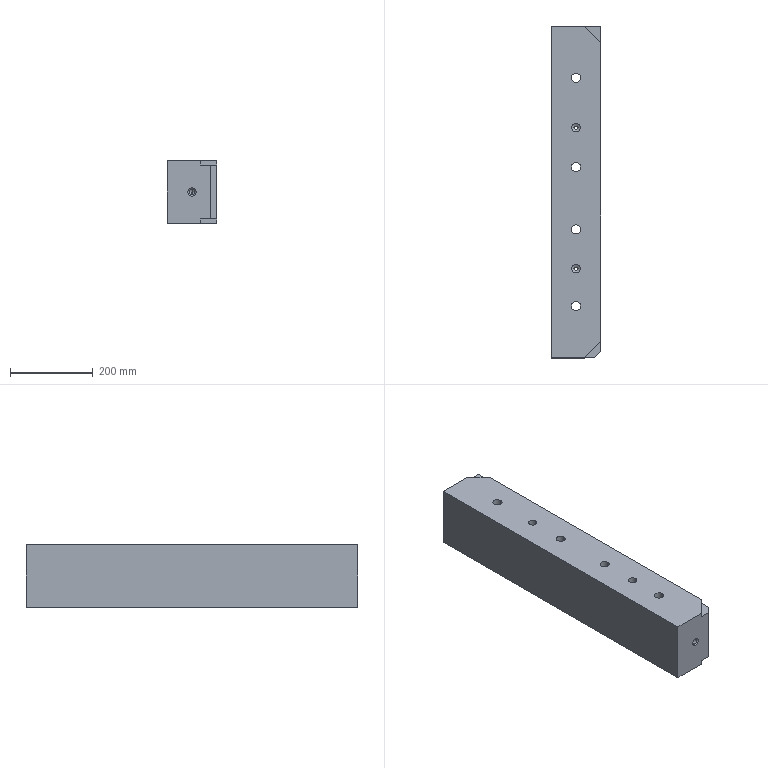Part | Creo | 1 solid | 63 faces | box 120 x 800 x 150 mm | volume 14052045 mm3 | cylinder 28 | cone 20 | plane 15 | commonest cylinder face diameters 20 x8 22 x8 8 x4 12 x4 14 x4